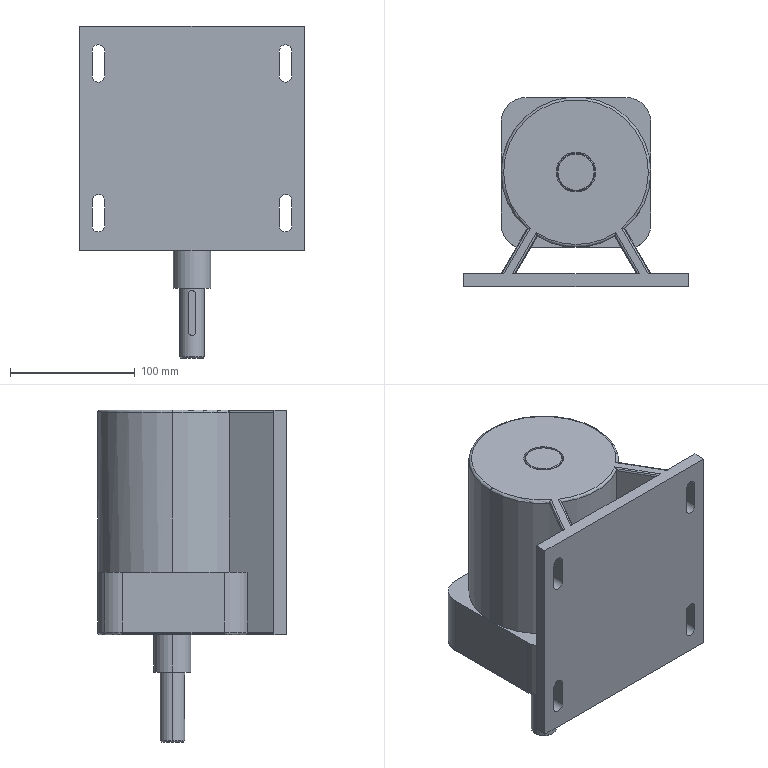Part | SolidWorks | features BaseBody 1 | 1 solid | 124 faces | box 180 x 151.384 x 266 mm | volume 2647697 mm3 | cylinder 66 | plane 40 | torus 16 | cone 2 | commonest cylinder face diameters 4 x24 10 x16 40 x8 30 x4 120 x4 6 x2